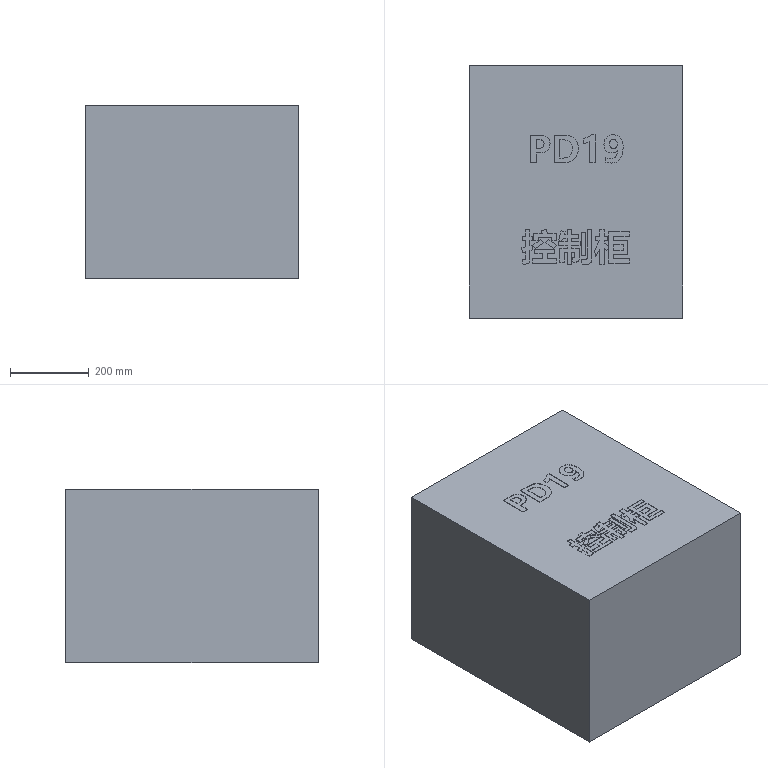Part | STEP file | PD19 | 1 solid | 207 faces | box 542 x 640 x 441 mm | volume 152648654 mm3 | plane 159 | spline 48